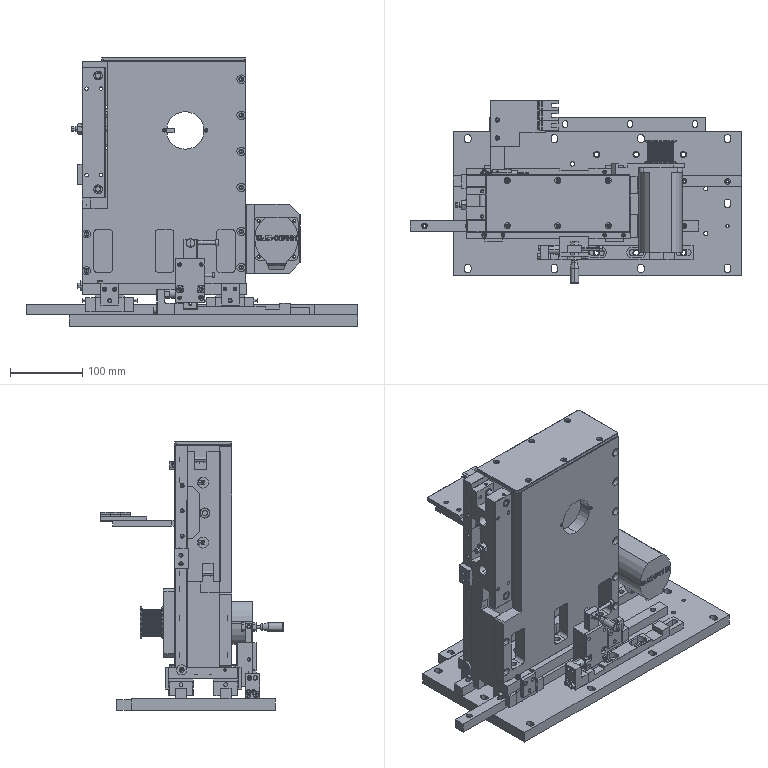Part | NX | 74 solids | 4373 faces | volume 5118134 mm3 | plane 2214 | cylinder 1473 | cone 632 | spline 44 | sphere 6 | torus 4 | commonest cylinder face diameters 5 x427 3.3 x150 4.5 x64 6.6 x54 0.5 x52 6.55 x52